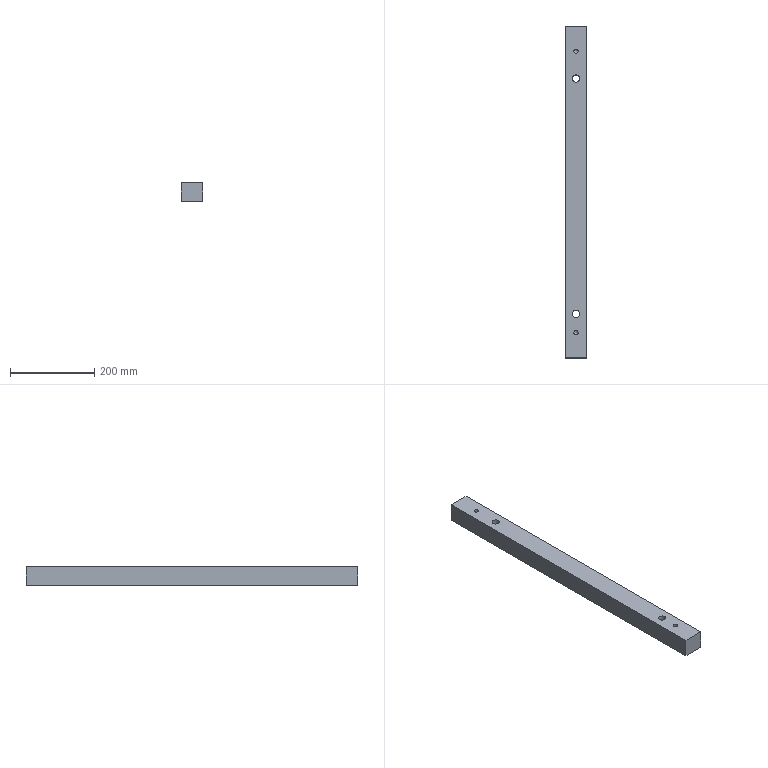Part | STEP file | 021_id2210_x_t | 1 solid | 16 faces | box 50 x 790 x 45 mm | volume 1744458 mm3 | plane 6 | cylinder 6 | cone 4 | commonest cylinder face diameters 10.3 x2 14 x2 17 x2
STEP:
#1=CARTESIAN_POINT('',(0.,0.,0.));
#2=DIRECTION('',(0.,0.,1.));
#3=DIRECTION('',(1.,0.,0.));
#4=AXIS2_PLACEMENT_3D('',#1,#2,#3);
#5=CARTESIAN_POINT('',(328.5,395.,185.));
#6=VERTEX_POINT('',#5);
#7=CARTESIAN_POINT('',(378.5,395.,185.));
#8=VERTEX_POINT('',#7);
#9=CARTESIAN_POINT('',(533.5,395.,185.));
#10=DIRECTION('',(1.,0.,0.));
#11=VECTOR('',#10,1.);
#12=LINE('',#9,#11);
#13=CARTESIAN_POINT('',(533.5,0.,185.));
#14=DIRECTION('',(0.,0.,-1.));
#15=DIRECTION('',(1.,0.,0.));
#16=AXIS2_PLACEMENT_3D('',#13,#14,#15);
#17=PLANE('',#16);
#18=CARTESIAN_POINT('',(0.,-395.));
#19=DIRECTION('',(1.,0.));
#20=VECTOR('',#19,1.);
#21=LINE('',#18,#20);
#22=(GEOMETRIC_REPRESENTATION_CONTEXT(2)PARAMETRIC_REPRESENTATION_CONTEXT()REPRESENTATION_CONTEXT('',''));
#23=DEFINITIONAL_REPRESENTATION('',(#21),#22);
#24=PCURVE('',#17,#23);
#25=CARTESIAN_POINT('',(328.5,395.,-28.5));
#26=DIRECTION('',(0.,1.,0.));
#27=DIRECTION('',(0.,0.,-1.));
#28=AXIS2_PLACEMENT_3D('',#25,#26,#27);
#29=PLANE('',#28);
#30=CARTESIAN_POINT('',(-213.5,-205.));
#31=DIRECTION('',(0.,-1.));
#32=VECTOR('',#31,1.);
#33=LINE('',#30,#32);
#34=(GEOMETRIC_REPRESENTATION_CONTEXT(2)PARAMETRIC_REPRESENTATION_CONTEXT()REPRESENTATION_CONTEXT('',''));
#35=DEFINITIONAL_REPRESENTATION('',(#33),#34);
#36=PCURVE('',#29,#35);
#37=SURFACE_CURVE('',#12,(#24,#36),.PCURVE_S1.);
#38=EDGE_CURVE('',#6,#8,#37,.T.);
#39=ORIENTED_EDGE('',*,*,#38,.T.);
#40=CARTESIAN_POINT('',(378.5,-395.,185.));
#41=VERTEX_POINT('',#40);
#42=CARTESIAN_POINT('',(378.5,-210.,185.));
#43=DIRECTION('',(0.,-1.,0.));
#44=VECTOR('',#43,1.);
#45=LINE('',#42,#44);
#46=CARTESIAN_POINT('',(-155.,210.));
#47=DIRECTION('',(0.,1.));
#48=VECTOR('',#47,1.);
#49=LINE('',#46,#48);
#50=(GEOMETRIC_REPRESENTATION_CONTEXT(2)PARAMETRIC_REPRESENTATION_CONTEXT()REPRESENTATION_CONTEXT('',''));
#51=DEFINITIONAL_REPRESENTATION('',(#49),#50);
#52=PCURVE('',#17,#51);
#53=CARTESIAN_POINT('',(378.5,-210.,-28.5));
#54=DIRECTION('',(-1.,0.,0.));
#55=DIRECTION('',(0.,0.,1.));
#56=AXIS2_PLACEMENT_3D('',#53,#54,#55);
#57=PLANE('',#56);
#58=CARTESIAN_POINT('',(213.5,0.));
#59=DIRECTION('',(0.,-1.));
#60=VECTOR('',#59,1.);
#61=LINE('',#58,#60);
#62=(GEOMETRIC_REPRESENTATION_CONTEXT(2)PARAMETRIC_REPRESENTATION_CONTEXT()REPRESENTATION_CONTEXT('',''));
#63=DEFINITIONAL_REPRESENTATION('',(#61),#62);
#64=PCURVE('',#57,#63);
#65=SURFACE_CURVE('',#45,(#52,#64),.PCURVE_S1.);
#66=EDGE_CURVE('',#8,#41,#65,.T.);
#67=ORIENTED_EDGE('',*,*,#66,.T.);
#68=CARTESIAN_POINT('',(328.5,-395.,185.));
#69=VERTEX_POINT('',#68);
#70=CARTESIAN_POINT('',(533.5,-395.,185.));
#71=DIRECTION('',(1.,0.,0.));
#72=VECTOR('',#71,1.);
#73=LINE('',#70,#72);
#74=CARTESIAN_POINT('',(0.,395.));
#75=DIRECTION('',(1.,0.));
#76=VECTOR('',#75,1.);
#77=LINE('',#74,#76);
#78=(GEOMETRIC_REPRESENTATION_CONTEXT(2)PARAMETRIC_REPRESENTATION_CONTEXT()REPRESENTATION_CONTEXT('',''));
#79=DEFINITIONAL_REPRESENTATION('',(#77),#78);
#80=PCURVE('',#17,#79);
#81=CARTESIAN_POINT('',(328.5,-395.,-28.5));
#82=DIRECTION('',(0.,1.,0.));
#83=DIRECTION('',(0.,0.,-1.));
#84=AXIS2_PLACEMENT_3D('',#81,#82,#83);
#85=PLANE('',#84);
#86=CARTESIAN_POINT('',(-213.5,-205.));
#87=DIRECTION('',(0.,-1.));
#88=VECTOR('',#87,1.);
#89=LINE('',#86,#88);
#90=(GEOMETRIC_REPRESENTATION_CONTEXT(2)PARAMETRIC_REPRESENTATION_CONTEXT()REPRESENTATION_CONTEXT('',''));
#91=DEFINITIONAL_REPRESENTATION('',(#89),#90);
#92=PCURVE('',#85,#91);
#93=SURFACE_CURVE('',#73,(#80,#92),.PCURVE_S1.);
#94=EDGE_CURVE('',#69,#41,#93,.T.);
#95=ORIENTED_EDGE('',*,*,#94,.F.);
#96=CARTESIAN_POINT('',(328.5,0.,185.));
#97=DIRECTION('',(0.,1.,0.));
#98=VECTOR('',#97,1.);
#99=LINE('',#96,#98);
#100=CARTESIAN_POINT('',(-205.,0.));
#101=DIRECTION('',(0.,-1.));
#102=VECTOR('',#101,1.);
#103=LINE('',#100,#102);
#104=(GEOMETRIC_REPRESENTATION_CONTEXT(2)PARAMETRIC_REPRESENTATION_CONTEXT()REPRESENTATION_CONTEXT('',''));
#105=DEFINITIONAL_REPRESENTATION('',(#103),#104);
#106=PCURVE('',#17,#105);
#107=CARTESIAN_POINT('',(328.5,-210.,-28.5));
#108=DIRECTION('',(-1.,0.,0.));
#109=DIRECTION('',(0.,0.,1.));
#110=AXIS2_PLACEMENT_3D('',#107,#108,#109);
#111=PLANE('',#110);
#112=CARTESIAN_POINT('',(213.5,210.));
#113=DIRECTION('',(0.,1.));
#114=VECTOR('',#113,1.);
#115=LINE('',#112,#114);
#116=(GEOMETRIC_REPRESENTATION_CONTEXT(2)PARAMETRIC_REPRESENTATION_CONTEXT()REPRESENTATION_CONTEXT('',''));
#117=DEFINITIONAL_REPRESENTATION('',(#115),#116);
#118=PCURVE('',#111,#117);
#119=SURFACE_CURVE('',#99,(#106,#118),.PCURVE_S1.);
#120=EDGE_CURVE('',#69,#6,#119,.T.);
#121=ORIENTED_EDGE('',*,*,#120,.T.);
#122=EDGE_LOOP('',(#39,#67,#95,#121));
#123=FACE_BOUND('',#122,.T.);
#124=CARTESIAN_POINT('',(346.5,-370.,185.));
#125=VERTEX_POINT('',#124);
#126=CARTESIAN_POINT('',(360.5,-370.,185.));
#127=VERTEX_POINT('',#126);
#128=CARTESIAN_POINT('',(353.5,-370.,185.));
#129=DIRECTION('',(0.,0.,1.));
#130=DIRECTION('',(-1.,0.,0.));
#131=AXIS2_PLACEMENT_3D('',#128,#129,#130);
#132=CIRCLE('',#131,7.);
#133=CARTESIAN_POINT('',(-187.,370.));
#134=CARTESIAN_POINT('',(-187.,382.124));
#135=CARTESIAN_POINT('',(-176.5,376.062));
#136=CARTESIAN_POINT('',(-166.,370.));
#137=CARTESIAN_POINT('',(-176.5,363.938));
#138=CARTESIAN_POINT('',(-187.,357.876));
#139=CARTESIAN_POINT('',(-187.,370.));
#140=(BOUNDED_CURVE()B_SPLINE_CURVE(2,(#133,#134,#135,#136,#137,#138,#139),.UNSPECIFIED.,.T.,.F.)B_SPLINE_CURVE_WITH_KNOTS((1,2,2,2,2,1),(-2.094,0.,2.094,4.189,6.283,8.378),.UNSPECIFIED.)CURVE()GEOMETRIC_REPRESENTATION_ITEM()RATIONAL_B_SPLINE_CURVE((1.,0.5,1.,0.5,1.,0.5,1.))REPRESENTATION_ITEM(''));
#141=(GEOMETRIC_REPRESENTATION_CONTEXT(2)PARAMETRIC_REPRESENTATION_CONTEXT()REPRESENTATION_CONTEXT('',''));
#142=DEFINITIONAL_REPRESENTATION('',(#140),#141);
#143=PCURVE('',#17,#142);
#144=CARTESIAN_POINT('',(353.5,-370.,121.));
#145=DIRECTION('',(0.,0.,1.));
#146=DIRECTION('',(1.,0.,0.));
#147=AXIS2_PLACEMENT_3D('',#144,#145,#146);
#148=CYLINDRICAL_SURFACE('',#147,7.);
#149=CARTESIAN_POINT('',(3.142,64.));
#150=DIRECTION('',(1.,0.));
#151=VECTOR('',#150,1.);
#152=LINE('',#149,#151);
#153=(GEOMETRIC_REPRESENTATION_CONTEXT(2)PARAMETRIC_REPRESENTATION_CONTEXT()REPRESENTATION_CONTEXT('',''));
#154=DEFINITIONAL_REPRESENTATION('',(#152),#153);
#155=PCURVE('',#148,#154);
#156=SURFACE_CURVE('',#132,(#143,#155),.PCURVE_S1.);
#157=EDGE_CURVE('',#125,#127,#156,.T.);
#158=ORIENTED_EDGE('',*,*,#157,.T.);
#159=CARTESIAN_POINT('',(353.5,-370.,185.));
#160=DIRECTION('',(0.,0.,1.));
#161=DIRECTION('',(-1.,0.,0.));
#162=AXIS2_PLACEMENT_3D('',#159,#160,#161);
#163=CIRCLE('',#162,7.);
#164=CARTESIAN_POINT('',(-187.,370.));
#165=CARTESIAN_POINT('',(-187.,382.124));
#166=CARTESIAN_POINT('',(-176.5,376.062));
#167=CARTESIAN_POINT('',(-166.,370.));
#168=CARTESIAN_POINT('',(-176.5,363.938));
#169=CARTESIAN_POINT('',(-187.,357.876));
#170=CARTESIAN_POINT('',(-187.,370.));
#171=(BOUNDED_CURVE()B_SPLINE_CURVE(2,(#164,#165,#166,#167,#168,#169,#170),.UNSPECIFIED.,.T.,.F.)B_SPLINE_CURVE_WITH_KNOTS((1,2,2,2,2,1),(-2.094,0.,2.094,4.189,6.283,8.378),.UNSPECIFIED.)CURVE()GEOMETRIC_REPRESENTATION_ITEM()RATIONAL_B_SPLINE_CURVE((1.,0.5,1.,0.5,1.,0.5,1.))REPRESENTATION_ITEM(''));
#172=(GEOMETRIC_REPRESENTATION_CONTEXT(2)PARAMETRIC_REPRESENTATION_CONTEXT()REPRESENTATION_CONTEXT('',''));
#173=DEFINITIONAL_REPRESENTATION('',(#171),#172);
#174=PCURVE('',#17,#173);
#175=CARTESIAN_POINT('',(-3.142,64.));
#176=DIRECTION('',(1.,0.));
#177=VECTOR('',#176,1.);
#178=LINE('',#175,#177);
#179=(GEOMETRIC_REPRESENTATION_CONTEXT(2)PARAMETRIC_REPRESENTATION_CONTEXT()REPRESENTATION_CONTEXT('',''));
#180=DEFINITIONAL_REPRESENTATION('',(#178),#179);
#181=PCURVE('',#148,#180);
#182=SURFACE_CURVE('',#163,(#174,#181),.PCURVE_S1.);
#183=EDGE_CURVE('',#127,#125,#182,.T.);
#184=ORIENTED_EDGE('',*,*,#183,.T.);
#185=EDGE_LOOP('',(#158,#184));
#186=FACE_BOUND('',#185,.T.);
#187=CARTESIAN_POINT('',(346.5,370.,185.));
#188=VERTEX_POINT('',#187);
#189=CARTESIAN_POINT('',(360.5,370.,185.));
#190=VERTEX_POINT('',#189);
#191=CARTESIAN_POINT('',(353.5,370.,185.));
#192=DIRECTION('',(0.,0.,-1.));
#193=DIRECTION('',(-1.,0.,0.));
#194=AXIS2_PLACEMENT_3D('',#191,#192,#193);
#195=CIRCLE('',#194,7.);
#196=CARTESIAN_POINT('',(-180.,-370.));
#197=DIRECTION('',(-1.,0.));
#198=AXIS2_PLACEMENT_2D('',#196,#197);
#199=CIRCLE('',#198,7.);
#200=(GEOMETRIC_REPRESENTATION_CONTEXT(2)PARAMETRIC_REPRESENTATION_CONTEXT()REPRESENTATION_CONTEXT('',''));
#201=DEFINITIONAL_REPRESENTATION('',(#199),#200);
#202=PCURVE('',#17,#201);
#203=CARTESIAN_POINT('',(353.5,370.,121.));
#204=DIRECTION('',(0.,0.,1.));
#205=DIRECTION('',(1.,0.,0.));
#206=AXIS2_PLACEMENT_3D('',#203,#204,#205);
#207=CYLINDRICAL_SURFACE('',#206,7.);
#208=CARTESIAN_POINT('',(3.142,64.));
#209=DIRECTION('',(-1.,0.));
#210=VECTOR('',#209,1.);
#211=LINE('',#208,#210);
#212=(GEOMETRIC_REPRESENTATION_CONTEXT(2)PARAMETRIC_REPRESENTATION_CONTEXT()REPRESENTATION_CONTEXT('',''));
#213=DEFINITIONAL_REPRESENTATION('',(#211),#212);
#214=PCURVE('',#207,#213);
#215=SURFACE_CURVE('',#195,(#202,#214),.PCURVE_S1.);
#216=EDGE_CURVE('',#188,#190,#215,.T.);
#217=ORIENTED_EDGE('',*,*,#216,.F.);
#218=CARTESIAN_POINT('',(353.5,370.,185.));
#219=DIRECTION('',(0.,0.,-1.));
#220=DIRECTION('',(-1.,0.,0.));
#221=AXIS2_PLACEMENT_3D('',#218,#219,#220);
#222=CIRCLE('',#221,7.);
#223=CARTESIAN_POINT('',(-180.,-370.));
#224=DIRECTION('',(-1.,0.));
#225=AXIS2_PLACEMENT_2D('',#223,#224);
#226=CIRCLE('',#225,7.);
#227=(GEOMETRIC_REPRESENTATION_CONTEXT(2)PARAMETRIC_REPRESENTATION_CONTEXT()REPRESENTATION_CONTEXT('',''));
#228=DEFINITIONAL_REPRESENTATION('',(#226),#227);
#229=PCURVE('',#17,#228);
#230=CARTESIAN_POINT('',(9.425,64.));
#231=DIRECTION('',(-1.,0.));
#232=VECTOR('',#231,1.);
#233=LINE('',#230,#232);
#234=(GEOMETRIC_REPRESENTATION_CONTEXT(2)PARAMETRIC_REPRESENTATION_CONTEXT()REPRESENTATION_CONTEXT('',''));
#235=DEFINITIONAL_REPRESENTATION('',(#233),#234);
#236=PCURVE('',#207,#235);
#237=SURFACE_CURVE('',#222,(#229,#236),.PCURVE_S1.);
#238=EDGE_CURVE('',#190,#188,#237,.T.);
#239=ORIENTED_EDGE('',*,*,#238,.F.);
#240=EDGE_LOOP('',(#217,#239));
#241=FACE_BOUND('',#240,.T.);
#242=CARTESIAN_POINT('',(345.,-290.,185.));
#243=VERTEX_POINT('',#242);
#244=CARTESIAN_POINT('',(353.5,-290.,185.));
#245=DIRECTION('',(0.,0.,-1.));
#246=DIRECTION('',(-1.,0.,0.));
#247=AXIS2_PLACEMENT_3D('',#244,#245,#246);
#248=CIRCLE('',#247,8.5);
#249=CARTESIAN_POINT('',(-180.,290.));
#250=DIRECTION('',(-1.,0.));
#251=AXIS2_PLACEMENT_2D('',#249,#250);
#252=CIRCLE('',#251,8.5);
#253=(GEOMETRIC_REPRESENTATION_CONTEXT(2)PARAMETRIC_REPRESENTATION_CONTEXT()REPRESENTATION_CONTEXT('',''));
#254=DEFINITIONAL_REPRESENTATION('',(#252),#253);
#255=PCURVE('',#17,#254);
#256=CARTESIAN_POINT('',(353.5,-290.,150.016));
#257=DIRECTION('',(0.,0.,1.));
#258=DIRECTION('',(1.,0.,0.));
#259=AXIS2_PLACEMENT_3D('',#256,#257,#258);
#260=CYLINDRICAL_SURFACE('',#259,8.5);
#261=CARTESIAN_POINT('',(9.425,34.984));
#262=DIRECTION('',(-1.,0.));
#263=VECTOR('',#262,1.);
#264=LINE('',#261,#263);
#265=(GEOMETRIC_REPRESENTATION_CONTEXT(2)PARAMETRIC_REPRESENTATION_CONTEXT()REPRESENTATION_CONTEXT('',''));
#266=DEFINITIONAL_REPRESENTATION('',(#264),#265);
#267=PCURVE('',#260,#266);
#268=SURFACE_CURVE('',#248,(#255,#267),.PCURVE_S1.);
#269=EDGE_CURVE('',#243,#243,#268,.T.);
#270=ORIENTED_EDGE('',*,*,#269,.F.);
#271=EDGE_LOOP('',(#270));
#272=FACE_BOUND('',#271,.T.);
#273=CARTESIAN_POINT('',(345.,270.,185.));
#274=VERTEX_POINT('',#273);
#275=CARTESIAN_POINT('',(353.5,270.,185.));
#276=DIRECTION('',(0.,0.,1.));
#277=DIRECTION('',(-1.,0.,0.));
#278=AXIS2_PLACEMENT_3D('',#275,#276,#277);
#279=CIRCLE('',#278,8.5);
#280=CARTESIAN_POINT('',(-188.5,-270.));
#281=CARTESIAN_POINT('',(-188.5,-255.278));
#282=CARTESIAN_POINT('',(-175.75,-262.639));
#283=CARTESIAN_POINT('',(-163.,-270.));
#284=CARTESIAN_POINT('',(-175.75,-277.361));
#285=CARTESIAN_POINT('',(-188.5,-284.722));
#286=CARTESIAN_POINT('',(-188.5,-270.));
#287=(BOUNDED_CURVE()B_SPLINE_CURVE(2,(#280,#281,#282,#283,#284,#285,#286),.UNSPECIFIED.,.T.,.F.)B_SPLINE_CURVE_WITH_KNOTS((1,2,2,2,2,1),(-2.094,0.,2.094,4.189,6.283,8.378),.UNSPECIFIED.)CURVE()GEOMETRIC_REPRESENTATION_ITEM()RATIONAL_B_SPLINE_CURVE((1.,0.5,1.,0.5,1.,0.5,1.))REPRESENTATION_ITEM(''));
#288=(GEOMETRIC_REPRESENTATION_CONTEXT(2)PARAMETRIC_REPRESENTATION_CONTEXT()REPRESENTATION_CONTEXT('',''));
#289=DEFINITIONAL_REPRESENTATION('',(#287),#288);
#290=PCURVE('',#17,#289);
#291=CARTESIAN_POINT('',(353.5,270.,150.016));
#292=DIRECTION('',(0.,0.,1.));
#293=DIRECTION('',(1.,0.,0.));
#294=AXIS2_PLACEMENT_3D('',#291,#292,#293);
#295=CYLINDRICAL_SURFACE('',#294,8.5);
#296=CARTESIAN_POINT('',(3.142,34.984));
#297=DIRECTION('',(1.,0.));
#298=VECTOR('',#297,1.);
#299=LINE('',#296,#298);
#300=(GEOMETRIC_REPRESENTATION_CONTEXT(2)PARAMETRIC_REPRESENTATION_CONTEXT()REPRESENTATION_CONTEXT('',''));
#301=DEFINITIONAL_REPRESENTATION('',(#299),#300);
#302=PCURVE('',#295,#301);
#303=SURFACE_CURVE('',#279,(#290,#302),.PCURVE_S1.);
#304=EDGE_CURVE('',#274,#274,#303,.T.);
#305=ORIENTED_EDGE('',*,*,#304,.T.);
#306=EDGE_LOOP('',(#305));
#307=FACE_BOUND('',#306,.T.);
#308=ADVANCED_FACE('',(#123,#186,#241,#272,#307),#17,.T.);
#309=CARTESIAN_POINT('',(348.35,-335.,230.));
#310=VERTEX_POINT('',#309);
#311=CARTESIAN_POINT('',(353.5,-335.,230.));
#312=DIRECTION('',(0.,0.,-1.));
#313=DIRECTION('',(-1.,0.,0.));
#314=AXIS2_PLACEMENT_3D('',#311,#312,#313);
#315=CIRCLE('',#314,5.15);
#316=CARTESIAN_POINT('',(328.5,-210.,230.));
#317=DIRECTION('',(0.,0.,-1.));
#318=DIRECTION('',(0.,-1.,0.));
#319=AXIS2_PLACEMENT_3D('',#316,#317,#318);
#320=PLANE('',#319);
#321=CARTESIAN_POINT('',(125.,-25.));
#322=DIRECTION('',(0.,1.));
#323=AXIS2_PLACEMENT_2D('',#321,#322);
#324=CIRCLE('',#323,5.15);
#325=(GEOMETRIC_REPRESENTATION_CONTEXT(2)PARAMETRIC_REPRESENTATION_CONTEXT()REPRESENTATION_CONTEXT('',''));
#326=DEFINITIONAL_REPRESENTATION('',(#324),#325);
#327=PCURVE('',#320,#326);
#328=CARTESIAN_POINT('',(353.5,-335.,259.));
#329=DIRECTION('',(0.,0.,-1.));
#330=DIRECTION('',(-1.,0.,0.));
#331=AXIS2_PLACEMENT_3D('',#328,#329,#330);
#332=CYLINDRICAL_SURFACE('',#331,5.15);
#333=CARTESIAN_POINT('',(0.,29.));
#334=DIRECTION('',(1.,0.));
#335=VECTOR('',#334,1.);
#336=LINE('',#333,#335);
#337=(GEOMETRIC_REPRESENTATION_CONTEXT(2)PARAMETRIC_REPRESENTATION_CONTEXT()REPRESENTATION_CONTEXT('',''));
#338=DEFINITIONAL_REPRESENTATION('',(#336),#337);
#339=PCURVE('',#332,#338);
#340=SURFACE_CURVE('',#315,(#327,#339),.PCURVE_S1.);
#341=EDGE_CURVE('',#310,#310,#340,.T.);
#342=ORIENTED_EDGE('',*,*,#341,.T.);
#343=EDGE_LOOP('',(#342));
#344=FACE_BOUND('',#343,.T.);
#345=CARTESIAN_POINT('',(348.35,335.,230.));
#346=VERTEX_POINT('',#345);
#347=CARTESIAN_POINT('',(353.5,335.,230.));
#348=DIRECTION('',(0.,0.,1.));
#349=DIRECTION('',(-1.,0.,0.));
#350=AXIS2_PLACEMENT_3D('',#347,#348,#349);
#351=CIRCLE('',#350,5.15);
#352=CARTESIAN_POINT('',(-545.,-19.85));
#353=CARTESIAN_POINT('',(-536.08,-19.85));
#354=CARTESIAN_POINT('',(-540.54,-27.575));
#355=CARTESIAN_POINT('',(-545.,-35.3));
#356=CARTESIAN_POINT('',(-549.46,-27.575));
#357=CARTESIAN_POINT('',(-553.92,-19.85));
#358=CARTESIAN_POINT('',(-545.,-19.85));
#359=(BOUNDED_CURVE()B_SPLINE_CURVE(2,(#352,#353,#354,#355,#356,#357,#358),.UNSPECIFIED.,.T.,.F.)B_SPLINE_CURVE_WITH_KNOTS((1,2,2,2,2,1),(-2.094,0.,2.094,4.189,6.283,8.378),.UNSPECIFIED.)CURVE()GEOMETRIC_REPRESENTATION_ITEM()RATIONAL_B_SPLINE_CURVE((1.,0.5,1.,0.5,1.,0.5,1.))REPRESENTATION_ITEM(''));
#360=(GEOMETRIC_REPRESENTATION_CONTEXT(2)PARAMETRIC_REPRESENTATION_CONTEXT()REPRESENTATION_CONTEXT('',''));
#361=DEFINITIONAL_REPRESENTATION('',(#359),#360);
#362=PCURVE('',#320,#361);
#363=CARTESIAN_POINT('',(353.5,335.,259.));
#364=DIRECTION('',(0.,0.,-1.));
#365=DIRECTION('',(-1.,0.,0.));
#366=AXIS2_PLACEMENT_3D('',#363,#364,#365);
#367=CYLINDRICAL_SURFACE('',#366,5.15);
#368=CARTESIAN_POINT('',(6.283,29.));
#369=DIRECTION('',(-1.,0.));
#370=VECTOR('',#369,1.);
#371=LINE('',#368,#370);
#372=(GEOMETRIC_REPRESENTATION_CONTEXT(2)PARAMETRIC_REPRESENTATION_CONTEXT()REPRESENTATION_CONTEXT('',''));
#373=DEFINITIONAL_REPRESENTATION('',(#371),#372);
#374=PCURVE('',#367,#373);
#375=SURFACE_CURVE('',#351,(#362,#374),.PCURVE_S1.);
#376=EDGE_CURVE('',#346,#346,#375,.T.);
#377=ORIENTED_EDGE('',*,*,#376,.F.);
#378=EDGE_LOOP('',(#377));
#379=FACE_BOUND('',#378,.T.);
#380=CARTESIAN_POINT('',(345.,270.,230.));
#381=VERTEX_POINT('',#380);
#382=CARTESIAN_POINT('',(353.5,270.,230.));
#383=DIRECTION('',(0.,0.,1.));
#384=DIRECTION('',(-1.,0.,0.));
#385=AXIS2_PLACEMENT_3D('',#382,#383,#384);
#386=CIRCLE('',#385,8.5);
#387=CARTESIAN_POINT('',(-480.,-16.5));
#388=CARTESIAN_POINT('',(-465.278,-16.5));
#389=CARTESIAN_POINT('',(-472.639,-29.25));
#390=CARTESIAN_POINT('',(-480.,-42.));
#391=CARTESIAN_POINT('',(-487.361,-29.25));
#392=CARTESIAN_POINT('',(-494.722,-16.5));
#393=CARTESIAN_POINT('',(-480.,-16.5));
#394=(BOUNDED_CURVE()B_SPLINE_CURVE(2,(#387,#388,#389,#390,#391,#392,#393),.UNSPECIFIED.,.T.,.F.)B_SPLINE_CURVE_WITH_KNOTS((1,2,2,2,2,1),(-2.094,0.,2.094,4.189,6.283,8.378),.UNSPECIFIED.)CURVE()GEOMETRIC_REPRESENTATION_ITEM()RATIONAL_B_SPLINE_CURVE((1.,0.5,1.,0.5,1.,0.5,1.))REPRESENTATION_ITEM(''));
#395=(GEOMETRIC_REPRESENTATION_CONTEXT(2)PARAMETRIC_REPRESENTATION_CONTEXT()REPRESENTATION_CONTEXT('',''));
#396=DEFINITIONAL_REPRESENTATION('',(#394),#395);
#397=PCURVE('',#320,#396);
#398=CARTESIAN_POINT('',(3.142,79.984));
#399=DIRECTION('',(1.,0.));
#400=VECTOR('',#399,1.);
#401=LINE('',#398,#400);
#402=(GEOMETRIC_REPRESENTATION_CONTEXT(2)PARAMETRIC_REPRESENTATION_CONTEXT()REPRESENTATION_CONTEXT('',''));
#403=DEFINITIONAL_REPRESENTATION('',(#401),#402);
#404=PCURVE('',#295,#403);
#405=SURFACE_CURVE('',#386,(#397,#404),.PCURVE_S1.);
#406=EDGE_CURVE('',#381,#381,#405,.T.);
#407=ORIENTED_EDGE('',*,*,#406,.F.);
#408=EDGE_LOOP('',(#407));
#409=FACE_BOUND('',#408,.T.);
#410=CARTESIAN_POINT('',(345.,-290.,230.));
#411=VERTEX_POINT('',#410);
#412=CARTESIAN_POINT('',(353.5,-290.,230.));
#413=DIRECTION('',(0.,0.,-1.));
#414=DIRECTION('',(-1.,0.,0.));
#415=AXIS2_PLACEMENT_3D('',#412,#413,#414);
#416=CIRCLE('',#415,8.5);
#417=CARTESIAN_POINT('',(80.,-25.));
#418=DIRECTION('',(0.,1.));
#419=AXIS2_PLACEMENT_2D('',#417,#418);
#420=CIRCLE('',#419,8.5);
#421=(GEOMETRIC_REPRESENTATION_CONTEXT(2)PARAMETRIC_REPRESENTATION_CONTEXT()REPRESENTATION_CONTEXT('',''));
#422=DEFINITIONAL_REPRESENTATION('',(#420),#421);
#423=PCURVE('',#320,#422);
#424=CARTESIAN_POINT('',(9.425,79.984));
#425=DIRECTION('',(-1.,0.));
#426=VECTOR('',#425,1.);
#427=LINE('',#424,#426);
#428=(GEOMETRIC_REPRESENTATION_CONTEXT(2)PARAMETRIC_REPRESENTATION_CONTEXT()REPRESENTATION_CONTEXT('',''));
#429=DEFINITIONAL_REPRESENTATION('',(#427),#428);
#430=PCURVE('',#260,#429);
#431=SURFACE_CURVE('',#416,(#423,#430),.PCURVE_S1.);
#432=EDGE_CURVE('',#411,#411,#431,.T.);
#433=ORIENTED_EDGE('',*,*,#432,.T.);
#434=EDGE_LOOP('',(#433));
#435=FACE_BOUND('',#434,.T.);
#436=CARTESIAN_POINT('',(328.5,-395.,230.));
#437=VERTEX_POINT('',#436);
#438=CARTESIAN_POINT('',(378.5,-395.,230.));
#439=VERTEX_POINT('',#438);
#440=CARTESIAN_POINT('',(328.5,-395.,230.));
#441=DIRECTION('',(1.,0.,0.));
#442=VECTOR('',#441,1.);
#443=LINE('',#440,#442);
#444=CARTESIAN_POINT('',(185.,0.));
#445=DIRECTION('',(0.,-1.));
#446=VECTOR('',#445,1.);
#447=LINE('',#444,#446);
#448=(GEOMETRIC_REPRESENTATION_CONTEXT(2)PARAMETRIC_REPRESENTATION_CONTEXT()REPRESENTATION_CONTEXT('',''));
#449=DEFINITIONAL_REPRESENTATION('',(#447),#448);
#450=PCURVE('',#320,#449);
#451=CARTESIAN_POINT('',(-258.5,0.));
#452=DIRECTION('',(0.,-1.));
#453=VECTOR('',#452,1.);
#454=LINE('',#451,#453);
#455=(GEOMETRIC_REPRESENTATION_CONTEXT(2)PARAMETRIC_REPRESENTATION_CONTEXT()REPRESENTATION_CONTEXT('',''));
#456=DEFINITIONAL_REPRESENTATION('',(#454),#455);
#457=PCURVE('',#85,#456);
#458=SURFACE_CURVE('',#443,(#450,#457),.PCURVE_S1.);
#459=EDGE_CURVE('',#437,#439,#458,.T.);
#460=ORIENTED_EDGE('',*,*,#459,.T.);
#461=CARTESIAN_POINT('',(378.5,395.,230.));
#462=VERTEX_POINT('',#461);
#463=CARTESIAN_POINT('',(378.5,-210.,230.));
#464=DIRECTION('',(0.,-1.,0.));
#465=VECTOR('',#464,1.);
#466=LINE('',#463,#465);
#467=CARTESIAN_POINT('',(0.,-50.));
#468=DIRECTION('',(1.,0.));
#469=VECTOR('',#468,1.);
#470=LINE('',#467,#469);
#471=(GEOMETRIC_REPRESENTATION_CONTEXT(2)PARAMETRIC_REPRESENTATION_CONTEXT()REPRESENTATION_CONTEXT('',''));
#472=DEFINITIONAL_REPRESENTATION('',(#470),#471);
#473=PCURVE('',#320,#472);
#474=CARTESIAN_POINT('',(258.5,0.));
#475=DIRECTION('',(0.,-1.));
#476=VECTOR('',#475,1.);
#477=LINE('',#474,#476);
#478=(GEOMETRIC_REPRESENTATION_CONTEXT(2)PARAMETRIC_REPRESENTATION_CONTEXT()REPRESENTATION_CONTEXT('',''));
#479=DEFINITIONAL_REPRESENTATION('',(#477),#478);
#480=PCURVE('',#57,#479);
#481=SURFACE_CURVE('',#466,(#473,#480),.PCURVE_S1.);
#482=EDGE_CURVE('',#462,#439,#481,.T.);
#483=ORIENTED_EDGE('',*,*,#482,.F.);
#484=CARTESIAN_POINT('',(328.5,395.,230.));
#485=VERTEX_POINT('',#484);
#486=CARTESIAN_POINT('',(328.5,395.,230.));
#487=DIRECTION('',(1.,0.,0.));
#488=VECTOR('',#487,1.);
#489=LINE('',#486,#488);
#490=CARTESIAN_POINT('',(-605.,0.));
#491=DIRECTION('',(0.,-1.));
#492=VECTOR('',#491,1.);
#493=LINE('',#490,#492);
#494=(GEOMETRIC_REPRESENTATION_CONTEXT(2)PARAMETRIC_REPRESENTATION_CONTEXT()REPRESENTATION_CONTEXT('',''));
#495=DEFINITIONAL_REPRESENTATION('',(#493),#494);
#496=PCURVE('',#320,#495);
#497=CARTESIAN_POINT('',(-258.5,0.));
#498=DIRECTION('',(0.,-1.));
#499=VECTOR('',#498,1.);
#500=LINE('',#497,#499);
#501=(GEOMETRIC_REPRESENTATION_CONTEXT(2)PARAMETRIC_REPRESENTATION_CONTEXT()REPRESENTATION_CONTEXT('',''));
#502=DEFINITIONAL_REPRESENTATION('',(#500),#501);
#503=PCURVE('',#29,#502);
#504=SURFACE_CURVE('',#489,(#496,#503),.PCURVE_S1.);
#505=EDGE_CURVE('',#485,#462,#504,.T.);
#506=ORIENTED_EDGE('',*,*,#505,.F.);
#507=CARTESIAN_POINT('',(328.5,-210.,230.));
#508=DIRECTION('',(0.,-1.,0.));
#509=VECTOR('',#508,1.);
#510=LINE('',#507,#509);
#511=CARTESIAN_POINT('',(0.,0.));
#512=DIRECTION('',(1.,0.));
#513=VECTOR('',#512,1.);
#514=LINE('',#511,#513);
#515=(GEOMETRIC_REPRESENTATION_CONTEXT(2)PARAMETRIC_REPRESENTATION_CONTEXT()REPRESENTATION_CONTEXT('',''));
#516=DEFINITIONAL_REPRESENTATION('',(#514),#515);
#517=PCURVE('',#320,#516);
#518=CARTESIAN_POINT('',(258.5,0.));
#519=DIRECTION('',(0.,-1.));
#520=VECTOR('',#519,1.);
#521=LINE('',#518,#520);
#522=(GEOMETRIC_REPRESENTATION_CONTEXT(2)PARAMETRIC_REPRESENTATION_CONTEXT()REPRESENTATION_CONTEXT('',''));
#523=DEFINITIONAL_REPRESENTATION('',(#521),#522);
#524=PCURVE('',#111,#523);
#525=SURFACE_CURVE('',#510,(#517,#524),.PCURVE_S1.);
#526=EDGE_CURVE('',#485,#437,#525,.T.);
#527=ORIENTED_EDGE('',*,*,#526,.T.);
#528=EDGE_LOOP('',(#460,#483,#506,#527));
#529=FACE_BOUND('',#528,.T.);
#530=ADVANCED_FACE('',(#344,#379,#409,#435,#529),#320,.F.);
#531=ORIENTED_EDGE('',*,*,#66,.F.);
#532=CARTESIAN_POINT('',(378.5,395.,-28.5));
#533=DIRECTION('',(0.,0.,1.));
#534=VECTOR('',#533,1.);
#535=LINE('',#532,#534);
#536=CARTESIAN_POINT('',(0.,605.));
#537=DIRECTION('',(1.,0.));
#538=VECTOR('',#537,1.);
#539=LINE('',#536,#538);
#540=(GEOMETRIC_REPRESENTATION_CONTEXT(2)PARAMETRIC_REPRESENTATION_CONTEXT()REPRESENTATION_CONTEXT('',''));
#541=DEFINITIONAL_REPRESENTATION('',(#539),#540);
#542=PCURVE('',#57,#541);
#543=CARTESIAN_POINT('',(0.,-50.));
#544=DIRECTION('',(-1.,0.));
#545=VECTOR('',#544,1.);
#546=LINE('',#543,#545);
#547=(GEOMETRIC_REPRESENTATION_CONTEXT(2)PARAMETRIC_REPRESENTATION_CONTEXT()REPRESENTATION_CONTEXT('',''));
#548=DEFINITIONAL_REPRESENTATION('',(#546),#547);
#549=PCURVE('',#29,#548);
#550=SURFACE_CURVE('',#535,(#542,#549),.PCURVE_S1.);
#551=EDGE_CURVE('',#8,#462,#550,.T.);
#552=ORIENTED_EDGE('',*,*,#551,.T.);
#553=ORIENTED_EDGE('',*,*,#482,.T.);
#554=CARTESIAN_POINT('',(378.5,-395.,-28.5));
#555=DIRECTION('',(0.,0.,-1.));
#556=VECTOR('',#555,1.);
#557=LINE('',#554,#556);
#558=CARTESIAN_POINT('',(0.,-185.));
#559=DIRECTION('',(-1.,0.));
#560=VECTOR('',#559,1.);
#561=LINE('',#558,#560);
#562=(GEOMETRIC_REPRESENTATION_CONTEXT(2)PARAMETRIC_REPRESENTATION_CONTEXT()REPRESENTATION_CONTEXT('',''));
#563=DEFINITIONAL_REPRESENTATION('',(#561),#562);
#564=PCURVE('',#57,#563);
#565=CARTESIAN_POINT('',(0.,-50.));
#566=DIRECTION('',(1.,0.));
#567=VECTOR('',#566,1.);
#568=LINE('',#565,#567);
#569=(GEOMETRIC_REPRESENTATION_CONTEXT(2)PARAMETRIC_REPRESENTATION_CONTEXT()REPRESENTATION_CONTEXT('',''));
#570=DEFINITIONAL_REPRESENTATION('',(#568),#569);
#571=PCURVE('',#85,#570);
#572=SURFACE_CURVE('',#557,(#564,#571),.PCURVE_S1.);
#573=EDGE_CURVE('',#439,#41,#572,.T.);
#574=ORIENTED_EDGE('',*,*,#573,.T.);
#575=EDGE_LOOP('',(#531,#552,#553,#574));
#576=FACE_BOUND('',#575,.T.);
#577=ADVANCED_FACE('',(#576),#57,.F.);
#578=ORIENTED_EDGE('',*,*,#94,.T.);
#579=ORIENTED_EDGE('',*,*,#573,.F.);
#580=ORIENTED_EDGE('',*,*,#459,.F.);
#581=CARTESIAN_POINT('',(328.5,-395.,-28.5));
#582=DIRECTION('',(0.,0.,-1.));
#583=VECTOR('',#582,1.);
#584=LINE('',#581,#583);
#585=CARTESIAN_POINT('',(0.,0.));
#586=DIRECTION('',(1.,0.));
#587=VECTOR('',#586,1.);
#588=LINE('',#585,#587);
#589=(GEOMETRIC_REPRESENTATION_CONTEXT(2)PARAMETRIC_REPRESENTATION_CONTEXT()REPRESENTATION_CONTEXT('',''));
#590=DEFINITIONAL_REPRESENTATION('',(#588),#589);
#591=PCURVE('',#85,#590);
#592=CARTESIAN_POINT('',(0.,-185.));
#593=DIRECTION('',(-1.,0.));
#594=VECTOR('',#593,1.);
#595=LINE('',#592,#594);
#596=(GEOMETRIC_REPRESENTATION_CONTEXT(2)PARAMETRIC_REPRESENTATION_CONTEXT()REPRESENTATION_CONTEXT('',''));
#597=DEFINITIONAL_REPRESENTATION('',(#595),#596);
#598=PCURVE('',#111,#597);
#599=SURFACE_CURVE('',#584,(#591,#598),.PCURVE_S1.);
#600=EDGE_CURVE('',#437,#69,#599,.T.);
#601=ORIENTED_EDGE('',*,*,#600,.T.);
#602=EDGE_LOOP('',(#578,#579,#580,#601));
#603=FACE_BOUND('',#602,.T.);
#604=ADVANCED_FACE('',(#603),#85,.F.);
#605=CARTESIAN_POINT('',(328.5,395.,-28.5));
#606=DIRECTION('',(0.,0.,1.));
#607=VECTOR('',#606,1.);
#608=LINE('',#605,#607);
#609=CARTESIAN_POINT('',(0.,605.));
#610=DIRECTION('',(1.,0.));
#611=VECTOR('',#610,1.);
#612=LINE('',#609,#611);
#613=(GEOMETRIC_REPRESENTATION_CONTEXT(2)PARAMETRIC_REPRESENTATION_CONTEXT()REPRESENTATION_CONTEXT('',''));
#614=DEFINITIONAL_REPRESENTATION('',(#612),#613);
#615=PCURVE('',#111,#614);
#616=CARTESIAN_POINT('',(0.,0.));
#617=DIRECTION('',(-1.,0.));
#618=VECTOR('',#617,1.);
#619=LINE('',#616,#618);
#620=(GEOMETRIC_REPRESENTATION_CONTEXT(2)PARAMETRIC_REPRESENTATION_CONTEXT()REPRESENTATION_CONTEXT('',''));
#621=DEFINITIONAL_REPRESENTATION('',(#619),#620);
#622=PCURVE('',#29,#621);
#623=SURFACE_CURVE('',#608,(#615,#622),.PCURVE_S1.);
#624=EDGE_CURVE('',#6,#485,#623,.T.);
#625=ORIENTED_EDGE('',*,*,#624,.F.);
#626=ORIENTED_EDGE('',*,*,#120,.F.);
#627=ORIENTED_EDGE('',*,*,#600,.F.);
#628=ORIENTED_EDGE('',*,*,#526,.F.);
#629=EDGE_LOOP('',(#625,#626,#627,#628));
#630=FACE_BOUND('',#629,.T.);
#631=ADVANCED_FACE('',(#630),#111,.T.);
#632=ORIENTED_EDGE('',*,*,#551,.F.);
#633=ORIENTED_EDGE('',*,*,#38,.F.);
#634=ORIENTED_EDGE('',*,*,#624,.T.);
#635=ORIENTED_EDGE('',*,*,#505,.T.);
#636=EDGE_LOOP('',(#632,#633,#634,#635));
#637=FACE_BOUND('',#636,.T.);
#638=ADVANCED_FACE('',(#637),#29,.T.);
#639=ORIENTED_EDGE('',*,*,#238,.F.);
#640=CARTESIAN_POINT('',(360.5,370.,209.459));
#641=VERTEX_POINT('',#640);
#642=CARTESIAN_POINT('',(360.5,370.,185.));
#643=CARTESIAN_POINT('',(360.5,370.,209.459));
#644=B_SPLINE_CURVE_WITH_KNOTS('',1,(#642,#643),.UNSPECIFIED.,.F.,.F.,(2,2),(64.,88.459),.PIECEWISE_BEZIER_KNOTS.);
#645=CARTESIAN_POINT('',(6.283,0.));
#646=DIRECTION('',(0.,1.));
#647=VECTOR('',#646,1.);
#648=LINE('',#645,#647);
#649=(GEOMETRIC_REPRESENTATION_CONTEXT(2)PARAMETRIC_REPRESENTATION_CONTEXT()REPRESENTATION_CONTEXT('',''));
#650=DEFINITIONAL_REPRESENTATION('',(#648),#649);
#651=PCURVE('',#207,#650);
#652=CARTESIAN_POINT('',(0.,0.));
#653=DIRECTION('',(0.,1.));
#654=VECTOR('',#653,1.);
#655=LINE('',#652,#654);
#656=(GEOMETRIC_REPRESENTATION_CONTEXT(2)PARAMETRIC_REPRESENTATION_CONTEXT()REPRESENTATION_CONTEXT('',''));
#657=DEFINITIONAL_REPRESENTATION('',(#655),#656);
#658=PCURVE('',#207,#657);
#659=SEAM_CURVE('',#644,(#651,#658),.PCURVE_S1.);
#660=EDGE_CURVE('',#190,#641,#659,.T.);
#661=ORIENTED_EDGE('',*,*,#660,.T.);
#662=CARTESIAN_POINT('',(346.5,370.,209.459));
#663=VERTEX_POINT('',#662);
#664=CARTESIAN_POINT('',(353.5,370.,209.459));
#665=DIRECTION('',(0.,0.,-1.));
#666=DIRECTION('',(1.,0.,0.));
#667=AXIS2_PLACEMENT_3D('',#664,#665,#666);
#668=CIRCLE('',#667,7.);
#669=CARTESIAN_POINT('',(6.283,88.459));
#670=DIRECTION('',(-1.,0.));
#671=VECTOR('',#670,1.);
#672=LINE('',#669,#671);
#673=(GEOMETRIC_REPRESENTATION_CONTEXT(2)PARAMETRIC_REPRESENTATION_CONTEXT()REPRESENTATION_CONTEXT('',''));
#674=DEFINITIONAL_REPRESENTATION('',(#672),#673);
#675=PCURVE('',#207,#674);
#676=CARTESIAN_POINT('',(353.5,370.,209.459));
#677=DIRECTION('',(0.,0.,-1.));
#678=DIRECTION('',(-1.,0.,0.));
#679=AXIS2_PLACEMENT_3D('',#676,#677,#678);
#680=CONICAL_SURFACE('',#679,7.,1.047);
#681=CARTESIAN_POINT('',(3.142,0.));
#682=DIRECTION('',(1.,0.));
#683=VECTOR('',#682,1.);
#684=LINE('',#681,#683);
#685=(GEOMETRIC_REPRESENTATION_CONTEXT(2)PARAMETRIC_REPRESENTATION_CONTEXT()REPRESENTATION_CONTEXT('',''));
#686=DEFINITIONAL_REPRESENTATION('',(#684),#685);
#687=PCURVE('',#680,#686);
#688=SURFACE_CURVE('',#668,(#675,#687),.PCURVE_S1.);
#689=EDGE_CURVE('',#641,#663,#688,.T.);
#690=ORIENTED_EDGE('',*,*,#689,.T.);
#691=CARTESIAN_POINT('',(353.5,370.,209.459));
#692=DIRECTION('',(0.,0.,-1.));
#693=DIRECTION('',(1.,0.,0.));
#694=AXIS2_PLACEMENT_3D('',#691,#692,#693);
#695=CIRCLE('',#694,7.);
#696=CARTESIAN_POINT('',(6.283,88.459));
#697=DIRECTION('',(-1.,0.));
#698=VECTOR('',#697,1.);
#699=LINE('',#696,#698);
#700=(GEOMETRIC_REPRESENTATION_CONTEXT(2)PARAMETRIC_REPRESENTATION_CONTEXT()REPRESENTATION_CONTEXT('',''));
#701=DEFINITIONAL_REPRESENTATION('',(#699),#700);
#702=PCURVE('',#207,#701);
#703=CARTESIAN_POINT('',(-3.142,0.));
#704=DIRECTION('',(1.,0.));
#705=VECTOR('',#704,1.);
#706=LINE('',#703,#705);
#707=(GEOMETRIC_REPRESENTATION_CONTEXT(2)PARAMETRIC_REPRESENTATION_CONTEXT()REPRESENTATION_CONTEXT('',''));
#708=DEFINITIONAL_REPRESENTATION('',(#706),#707);
#709=PCURVE('',#680,#708);
#710=SURFACE_CURVE('',#695,(#702,#709),.PCURVE_S1.);
#711=EDGE_CURVE('',#663,#641,#710,.T.);
#712=ORIENTED_EDGE('',*,*,#711,.T.);
#713=ORIENTED_EDGE('',*,*,#660,.F.);
#714=ORIENTED_EDGE('',*,*,#216,.F.);
#715=EDGE_LOOP('',(#639,#661,#690,#712,#713,#714));
#716=FACE_BOUND('',#715,.F.);
#717=ADVANCED_FACE('',(#716),#207,.F.);
#718=CARTESIAN_POINT('',(353.5,370.,213.5));
#719=VERTEX_POINT('',#718);
#720=CARTESIAN_POINT('',(353.5,370.,213.5));
#721=CARTESIAN_POINT('',(346.5,370.,209.459));
#722=B_SPLINE_CURVE_WITH_KNOTS('',1,(#720,#721),.UNSPECIFIED.,.F.,.F.,(2,2),(-8.083,0.),.PIECEWISE_BEZIER_KNOTS.);
#723=CARTESIAN_POINT('',(6.283,0.));
#724=DIRECTION('',(0.,1.));
#725=VECTOR('',#724,1.);
#726=LINE('',#723,#725);
#727=(GEOMETRIC_REPRESENTATION_CONTEXT(2)PARAMETRIC_REPRESENTATION_CONTEXT()REPRESENTATION_CONTEXT('',''));
#728=DEFINITIONAL_REPRESENTATION('',(#726),#727);
#729=PCURVE('',#680,#728);
#730=CARTESIAN_POINT('',(0.,0.));
#731=DIRECTION('',(0.,1.));
#732=VECTOR('',#731,1.);
#733=LINE('',#730,#732);
#734=(GEOMETRIC_REPRESENTATION_CONTEXT(2)PARAMETRIC_REPRESENTATION_CONTEXT()REPRESENTATION_CONTEXT('',''));
#735=DEFINITIONAL_REPRESENTATION('',(#733),#734);
#736=PCURVE('',#680,#735);
#737=SEAM_CURVE('',#722,(#729,#736),.PCURVE_S1.);
#738=EDGE_CURVE('',#719,#663,#737,.T.);
#739=ORIENTED_EDGE('',*,*,#738,.T.);
#740=ORIENTED_EDGE('',*,*,#689,.F.);
#741=ORIENTED_EDGE('',*,*,#711,.F.);
#742=ORIENTED_EDGE('',*,*,#738,.F.);
#743=EDGE_LOOP('',(#739,#740,#741,#742));
#744=FACE_BOUND('',#743,.F.);
#745=ADVANCED_FACE('',(#744),#680,.F.);
#746=ORIENTED_EDGE('',*,*,#157,.T.);
#747=CARTESIAN_POINT('',(360.5,-370.,209.459));
#748=VERTEX_POINT('',#747);
#749=CARTESIAN_POINT('',(360.5,-370.,185.));
#750=CARTESIAN_POINT('',(360.5,-370.,209.459));
#751=B_SPLINE_CURVE_WITH_KNOTS('',1,(#749,#750),.UNSPECIFIED.,.F.,.F.,(2,2),(64.,88.459),.PIECEWISE_BEZIER_KNOTS.);
#752=CARTESIAN_POINT('',(6.283,0.));
#753=DIRECTION('',(0.,1.));
#754=VECTOR('',#753,1.);
#755=LINE('',#752,#754);
#756=(GEOMETRIC_REPRESENTATION_CONTEXT(2)PARAMETRIC_REPRESENTATION_CONTEXT()REPRESENTATION_CONTEXT('',''));
#757=DEFINITIONAL_REPRESENTATION('',(#755),#756);
#758=PCURVE('',#148,#757);
#759=CARTESIAN_POINT('',(0.,0.));
#760=DIRECTION('',(0.,1.));
#761=VECTOR('',#760,1.);
#762=LINE('',#759,#761);
#763=(GEOMETRIC_REPRESENTATION_CONTEXT(2)PARAMETRIC_REPRESENTATION_CONTEXT()REPRESENTATION_CONTEXT('',''));
#764=DEFINITIONAL_REPRESENTATION('',(#762),#763);
#765=PCURVE('',#148,#764);
#766=SEAM_CURVE('',#751,(#758,#765),.PCURVE_S1.);
#767=EDGE_CURVE('',#127,#748,#766,.T.);
#768=ORIENTED_EDGE('',*,*,#767,.T.);
#769=CARTESIAN_POINT('',(346.5,-370.,209.459));
#770=VERTEX_POINT('',#769);
#771=CARTESIAN_POINT('',(353.5,-370.,209.459));
#772=DIRECTION('',(0.,0.,1.));
#773=DIRECTION('',(1.,0.,0.));
#774=AXIS2_PLACEMENT_3D('',#771,#772,#773);
#775=CIRCLE('',#774,7.);
#776=CARTESIAN_POINT('',(0.,88.459));
#777=DIRECTION('',(1.,0.));
#778=VECTOR('',#777,1.);
#779=LINE('',#776,#778);
#780=(GEOMETRIC_REPRESENTATION_CONTEXT(2)PARAMETRIC_REPRESENTATION_CONTEXT()REPRESENTATION_CONTEXT('',''));
#781=DEFINITIONAL_REPRESENTATION('',(#779),#780);
#782=PCURVE('',#148,#781);
#783=CARTESIAN_POINT('',(353.5,-370.,209.459));
#784=DIRECTION('',(0.,0.,-1.));
#785=DIRECTION('',(-1.,0.,0.));
#786=AXIS2_PLACEMENT_3D('',#783,#784,#785);
#787=CONICAL_SURFACE('',#786,7.,1.047);
#788=CARTESIAN_POINT('',(9.425,0.));
#789=DIRECTION('',(-1.,0.));
#790=VECTOR('',#789,1.);
#791=LINE('',#788,#790);
#792=(GEOMETRIC_REPRESENTATION_CONTEXT(2)PARAMETRIC_REPRESENTATION_CONTEXT()REPRESENTATION_CONTEXT('',''));
#793=DEFINITIONAL_REPRESENTATION('',(#791),#792);
#794=PCURVE('',#787,#793);
#795=SURFACE_CURVE('',#775,(#782,#794),.PCURVE_S1.);
#796=EDGE_CURVE('',#770,#748,#795,.T.);
#797=ORIENTED_EDGE('',*,*,#796,.F.);
#798=CARTESIAN_POINT('',(353.5,-370.,209.459));
#799=DIRECTION('',(0.,0.,1.));
#800=DIRECTION('',(1.,0.,0.));
#801=AXIS2_PLACEMENT_3D('',#798,#799,#800);
#802=CIRCLE('',#801,7.);
#803=CARTESIAN_POINT('',(0.,88.459));
#804=DIRECTION('',(1.,0.));
#805=VECTOR('',#804,1.);
#806=LINE('',#803,#805);
#807=(GEOMETRIC_REPRESENTATION_CONTEXT(2)PARAMETRIC_REPRESENTATION_CONTEXT()REPRESENTATION_CONTEXT('',''));
#808=DEFINITIONAL_REPRESENTATION('',(#806),#807);
#809=PCURVE('',#148,#808);
#810=CARTESIAN_POINT('',(3.142,0.));
#811=DIRECTION('',(-1.,0.));
#812=VECTOR('',#811,1.);
#813=LINE('',#810,#812);
#814=(GEOMETRIC_REPRESENTATION_CONTEXT(2)PARAMETRIC_REPRESENTATION_CONTEXT()REPRESENTATION_CONTEXT('',''));
#815=DEFINITIONAL_REPRESENTATION('',(#813),#814);
#816=PCURVE('',#787,#815);
#817=SURFACE_CURVE('',#802,(#809,#816),.PCURVE_S1.);
#818=EDGE_CURVE('',#748,#770,#817,.T.);
#819=ORIENTED_EDGE('',*,*,#818,.F.);
#820=ORIENTED_EDGE('',*,*,#767,.F.);
#821=ORIENTED_EDGE('',*,*,#183,.T.);
#822=EDGE_LOOP('',(#746,#768,#797,#819,#820,#821));
#823=FACE_BOUND('',#822,.F.);
#824=ADVANCED_FACE('',(#823),#148,.F.);
#825=CARTESIAN_POINT('',(353.5,-370.,213.5));
#826=VERTEX_POINT('',#825);
#827=CARTESIAN_POINT('',(353.5,-370.,213.5));
#828=CARTESIAN_POINT('',(346.5,-370.,209.459));
#829=B_SPLINE_CURVE_WITH_KNOTS('',1,(#827,#828),.UNSPECIFIED.,.F.,.F.,(2,2),(-8.083,0.),.PIECEWISE_BEZIER_KNOTS.);
#830=CARTESIAN_POINT('',(6.283,0.));
#831=DIRECTION('',(0.,1.));
#832=VECTOR('',#831,1.);
#833=LINE('',#830,#832);
#834=(GEOMETRIC_REPRESENTATION_CONTEXT(2)PARAMETRIC_REPRESENTATION_CONTEXT()REPRESENTATION_CONTEXT('',''));
#835=DEFINITIONAL_REPRESENTATION('',(#833),#834);
#836=PCURVE('',#787,#835);
#837=CARTESIAN_POINT('',(0.,0.));
#838=DIRECTION('',(0.,1.));
#839=VECTOR('',#838,1.);
#840=LINE('',#837,#839);
#841=(GEOMETRIC_REPRESENTATION_CONTEXT(2)PARAMETRIC_REPRESENTATION_CONTEXT()REPRESENTATION_CONTEXT('',''));
#842=DEFINITIONAL_REPRESENTATION('',(#840),#841);
#843=PCURVE('',#787,#842);
#844=SEAM_CURVE('',#829,(#836,#843),.PCURVE_S1.);
#845=EDGE_CURVE('',#826,#770,#844,.T.);
#846=ORIENTED_EDGE('',*,*,#845,.T.);
#847=ORIENTED_EDGE('',*,*,#796,.T.);
#848=ORIENTED_EDGE('',*,*,#818,.T.);
#849=ORIENTED_EDGE('',*,*,#845,.F.);
#850=EDGE_LOOP('',(#846,#847,#848,#849));
#851=FACE_BOUND('',#850,.F.);
#852=ADVANCED_FACE('',(#851),#787,.F.);
#853=ORIENTED_EDGE('',*,*,#269,.F.);
#854=CARTESIAN_POINT('',(345.,-290.,185.));
#855=CARTESIAN_POINT('',(345.,-290.,230.));
#856=B_SPLINE_CURVE_WITH_KNOTS('',1,(#854,#855),.UNSPECIFIED.,.F.,.F.,(2,2),(34.984,79.984),.PIECEWISE_BEZIER_KNOTS.);
#857=CARTESIAN_POINT('',(9.425,0.));
#858=DIRECTION('',(0.,1.));
#859=VECTOR('',#858,1.);
#860=LINE('',#857,#859);
#861=(GEOMETRIC_REPRESENTATION_CONTEXT(2)PARAMETRIC_REPRESENTATION_CONTEXT()REPRESENTATION_CONTEXT('',''));
#862=DEFINITIONAL_REPRESENTATION('',(#860),#861);
#863=PCURVE('',#260,#862);
#864=CARTESIAN_POINT('',(3.142,0.));
#865=DIRECTION('',(0.,1.));
#866=VECTOR('',#865,1.);
#867=LINE('',#864,#866);
#868=(GEOMETRIC_REPRESENTATION_CONTEXT(2)PARAMETRIC_REPRESENTATION_CONTEXT()REPRESENTATION_CONTEXT('',''));
#869=DEFINITIONAL_REPRESENTATION('',(#867),#868);
#870=PCURVE('',#260,#869);
#871=SEAM_CURVE('',#856,(#863,#870),.PCURVE_S1.);
#872=EDGE_CURVE('',#243,#411,#871,.T.);
#873=ORIENTED_EDGE('',*,*,#872,.T.);
#874=ORIENTED_EDGE('',*,*,#432,.T.);
#875=ORIENTED_EDGE('',*,*,#872,.F.);
#876=EDGE_LOOP('',(#853,#873,#874,#875));
#877=FACE_BOUND('',#876,.F.);
#878=ADVANCED_FACE('',(#877),#260,.F.);
#879=ORIENTED_EDGE('',*,*,#304,.T.);
#880=CARTESIAN_POINT('',(345.,270.,185.));
#881=CARTESIAN_POINT('',(345.,270.,230.));
#882=B_SPLINE_CURVE_WITH_KNOTS('',1,(#880,#881),.UNSPECIFIED.,.F.,.F.,(2,2),(34.984,79.984),.PIECEWISE_BEZIER_KNOTS.);
#883=CARTESIAN_POINT('',(9.425,0.));
#884=DIRECTION('',(0.,1.));
#885=VECTOR('',#884,1.);
#886=LINE('',#883,#885);
#887=(GEOMETRIC_REPRESENTATION_CONTEXT(2)PARAMETRIC_REPRESENTATION_CONTEXT()REPRESENTATION_CONTEXT('',''));
#888=DEFINITIONAL_REPRESENTATION('',(#886),#887);
#889=PCURVE('',#295,#888);
#890=CARTESIAN_POINT('',(3.142,0.));
#891=DIRECTION('',(0.,1.));
#892=VECTOR('',#891,1.);
#893=LINE('',#890,#892);
#894=(GEOMETRIC_REPRESENTATION_CONTEXT(2)PARAMETRIC_REPRESENTATION_CONTEXT()REPRESENTATION_CONTEXT('',''));
#895=DEFINITIONAL_REPRESENTATION('',(#893),#894);
#896=PCURVE('',#295,#895);
#897=SEAM_CURVE('',#882,(#889,#896),.PCURVE_S1.);
#898=EDGE_CURVE('',#274,#381,#897,.T.);
#899=ORIENTED_EDGE('',*,*,#898,.T.);
#900=ORIENTED_EDGE('',*,*,#406,.F.);
#901=ORIENTED_EDGE('',*,*,#898,.F.);
#902=EDGE_LOOP('',(#879,#899,#900,#901));
#903=FACE_BOUND('',#902,.F.);
#904=ADVANCED_FACE('',(#903),#295,.F.);
#905=ORIENTED_EDGE('',*,*,#376,.F.);
#906=CARTESIAN_POINT('',(348.35,335.,202.973));
#907=VERTEX_POINT('',#906);
#908=CARTESIAN_POINT('',(348.35,335.,230.));
#909=CARTESIAN_POINT('',(348.35,335.,202.973));
#910=B_SPLINE_CURVE_WITH_KNOTS('',1,(#908,#909),.UNSPECIFIED.,.F.,.F.,(2,2),(29.,56.027),.PIECEWISE_BEZIER_KNOTS.);
#911=CARTESIAN_POINT('',(6.283,0.));
#912=DIRECTION('',(0.,1.));
#913=VECTOR('',#912,1.);
#914=LINE('',#911,#913);
#915=(GEOMETRIC_REPRESENTATION_CONTEXT(2)PARAMETRIC_REPRESENTATION_CONTEXT()REPRESENTATION_CONTEXT('',''));
#916=DEFINITIONAL_REPRESENTATION('',(#914),#915);
#917=PCURVE('',#367,#916);
#918=CARTESIAN_POINT('',(0.,0.));
#919=DIRECTION('',(0.,1.));
#920=VECTOR('',#919,1.);
#921=LINE('',#918,#920);
#922=(GEOMETRIC_REPRESENTATION_CONTEXT(2)PARAMETRIC_REPRESENTATION_CONTEXT()REPRESENTATION_CONTEXT('',''));
#923=DEFINITIONAL_REPRESENTATION('',(#921),#922);
#924=PCURVE('',#367,#923);
#925=SEAM_CURVE('',#910,(#917,#924),.PCURVE_S1.);
#926=EDGE_CURVE('',#346,#907,#925,.T.);
#927=ORIENTED_EDGE('',*,*,#926,.T.);
#928=CARTESIAN_POINT('',(358.65,335.,202.973));
#929=VERTEX_POINT('',#928);
#930=CARTESIAN_POINT('',(353.5,335.,202.973));
#931=DIRECTION('',(0.,0.,1.));
#932=DIRECTION('',(1.,0.,0.));
#933=AXIS2_PLACEMENT_3D('',#930,#931,#932);
#934=CIRCLE('',#933,5.15);
#935=CARTESIAN_POINT('',(9.425,56.027));
#936=DIRECTION('',(-1.,0.));
#937=VECTOR('',#936,1.);
#938=LINE('',#935,#937);
#939=(GEOMETRIC_REPRESENTATION_CONTEXT(2)PARAMETRIC_REPRESENTATION_CONTEXT()REPRESENTATION_CONTEXT('',''));
#940=DEFINITIONAL_REPRESENTATION('',(#938),#939);
#941=PCURVE('',#367,#940);
#942=CARTESIAN_POINT('',(353.5,335.,202.944));
#943=DIRECTION('',(0.,0.,1.));
#944=DIRECTION('',(1.,0.,0.));
#945=AXIS2_PLACEMENT_3D('',#942,#943,#944);
#946=CONICAL_SURFACE('',#945,5.1,1.047);
#947=CARTESIAN_POINT('',(0.,0.02887));
#948=DIRECTION('',(1.,0.));
#949=VECTOR('',#948,1.);
#950=LINE('',#947,#949);
#951=(GEOMETRIC_REPRESENTATION_CONTEXT(2)PARAMETRIC_REPRESENTATION_CONTEXT()REPRESENTATION_CONTEXT('',''));
#952=DEFINITIONAL_REPRESENTATION('',(#950),#951);
#953=PCURVE('',#946,#952);
#954=SURFACE_CURVE('',#934,(#941,#953),.PCURVE_S1.);
#955=EDGE_CURVE('',#907,#929,#954,.T.);
#956=ORIENTED_EDGE('',*,*,#955,.T.);
#957=CARTESIAN_POINT('',(353.5,335.,202.973));
#958=DIRECTION('',(0.,0.,1.));
#959=DIRECTION('',(1.,0.,0.));
#960=AXIS2_PLACEMENT_3D('',#957,#958,#959);
#961=CIRCLE('',#960,5.15);
#962=CARTESIAN_POINT('',(3.142,56.027));
#963=DIRECTION('',(-1.,0.));
#964=VECTOR('',#963,1.);
#965=LINE('',#962,#964);
#966=(GEOMETRIC_REPRESENTATION_CONTEXT(2)PARAMETRIC_REPRESENTATION_CONTEXT()REPRESENTATION_CONTEXT('',''));
#967=DEFINITIONAL_REPRESENTATION('',(#965),#966);
#968=PCURVE('',#367,#967);
#969=CARTESIAN_POINT('',(0.,0.02887));
#970=DIRECTION('',(1.,0.));
#971=VECTOR('',#970,1.);
#972=LINE('',#969,#971);
#973=(GEOMETRIC_REPRESENTATION_CONTEXT(2)PARAMETRIC_REPRESENTATION_CONTEXT()REPRESENTATION_CONTEXT('',''));
#974=DEFINITIONAL_REPRESENTATION('',(#972),#973);
#975=PCURVE('',#946,#974);
#976=SURFACE_CURVE('',#961,(#968,#975),.PCURVE_S1.);
#977=EDGE_CURVE('',#929,#907,#976,.T.);
#978=ORIENTED_EDGE('',*,*,#977,.T.);
#979=ORIENTED_EDGE('',*,*,#926,.F.);
#980=EDGE_LOOP('',(#905,#927,#956,#978,#979));
#981=FACE_BOUND('',#980,.F.);
#982=ADVANCED_FACE('',(#981),#367,.F.);
#983=CARTESIAN_POINT('',(353.5,335.,200.));
#984=VERTEX_POINT('',#983);
#985=CARTESIAN_POINT('',(353.5,335.,200.));
#986=CARTESIAN_POINT('',(358.65,335.,202.973));
#987=B_SPLINE_CURVE_WITH_KNOTS('',1,(#985,#986),.UNSPECIFIED.,.F.,.F.,(2,2),(-5.889,0.05774),.PIECEWISE_BEZIER_KNOTS.);
#988=CARTESIAN_POINT('',(6.283,0.));
#989=DIRECTION('',(0.,1.));
#990=VECTOR('',#989,1.);
#991=LINE('',#988,#990);
#992=(GEOMETRIC_REPRESENTATION_CONTEXT(2)PARAMETRIC_REPRESENTATION_CONTEXT()REPRESENTATION_CONTEXT('',''));
#993=DEFINITIONAL_REPRESENTATION('',(#991),#992);
#994=PCURVE('',#946,#993);
#995=CARTESIAN_POINT('',(0.,0.));
#996=DIRECTION('',(0.,1.));
#997=VECTOR('',#996,1.);
#998=LINE('',#995,#997);
#999=(GEOMETRIC_REPRESENTATION_CONTEXT(2)PARAMETRIC_REPRESENTATION_CONTEXT()REPRESENTATION_CONTEXT('',''));
#1000=DEFINITIONAL_REPRESENTATION('',(#998),#999);
#1001=PCURVE('',#946,#1000);
#1002=SEAM_CURVE('',#987,(#994,#1001),.PCURVE_S1.);
#1003=EDGE_CURVE('',#984,#929,#1002,.T.);
#1004=ORIENTED_EDGE('',*,*,#1003,.T.);
#1005=ORIENTED_EDGE('',*,*,#955,.F.);
#1006=ORIENTED_EDGE('',*,*,#977,.F.);
#1007=ORIENTED_EDGE('',*,*,#1003,.F.);
#1008=EDGE_LOOP('',(#1004,#1005,#1006,#1007));
#1009=FACE_BOUND('',#1008,.F.);
#1010=ADVANCED_FACE('',(#1009),#946,.F.);
#1011=ORIENTED_EDGE('',*,*,#341,.T.);
#1012=CARTESIAN_POINT('',(348.35,-335.,202.973));
#1013=VERTEX_POINT('',#1012);
#1014=CARTESIAN_POINT('',(348.35,-335.,230.));
#1015=CARTESIAN_POINT('',(348.35,-335.,202.973));
#1016=B_SPLINE_CURVE_WITH_KNOTS('',1,(#1014,#1015),.UNSPECIFIED.,.F.,.F.,(2,2),(29.,56.027),.PIECEWISE_BEZIER_KNOTS.);
#1017=CARTESIAN_POINT('',(6.283,0.));
#1018=DIRECTION('',(0.,1.));
#1019=VECTOR('',#1018,1.);
#1020=LINE('',#1017,#1019);
#1021=(GEOMETRIC_REPRESENTATION_CONTEXT(2)PARAMETRIC_REPRESENTATION_CONTEXT()REPRESENTATION_CONTEXT('',''));
#1022=DEFINITIONAL_REPRESENTATION('',(#1020),#1021);
#1023=PCURVE('',#332,#1022);
#1024=CARTESIAN_POINT('',(0.,0.));
#1025=DIRECTION('',(0.,1.));
#1026=VECTOR('',#1025,1.);
#1027=LINE('',#1024,#1026);
#1028=(GEOMETRIC_REPRESENTATION_CONTEXT(2)PARAMETRIC_REPRESENTATION_CONTEXT()REPRESENTATION_CONTEXT('',''));
#1029=DEFINITIONAL_REPRESENTATION('',(#1027),#1028);
#1030=PCURVE('',#332,#1029);
#1031=SEAM_CURVE('',#1016,(#1023,#1030),.PCURVE_S1.);
#1032=EDGE_CURVE('',#310,#1013,#1031,.T.);
#1033=ORIENTED_EDGE('',*,*,#1032,.T.);
#1034=CARTESIAN_POINT('',(358.65,-335.,202.973));
#1035=VERTEX_POINT('',#1034);
#1036=CARTESIAN_POINT('',(353.5,-335.,202.973));
#1037=DIRECTION('',(0.,0.,-1.));
#1038=DIRECTION('',(1.,0.,0.));
#1039=AXIS2_PLACEMENT_3D('',#1036,#1037,#1038);
#1040=CIRCLE('',#1039,5.15);
#1041=CARTESIAN_POINT('',(3.142,56.027));
#1042=DIRECTION('',(1.,0.));
#1043=VECTOR('',#1042,1.);
#1044=LINE('',#1041,#1043);
#1045=(GEOMETRIC_REPRESENTATION_CONTEXT(2)PARAMETRIC_REPRESENTATION_CONTEXT()REPRESENTATION_CONTEXT('',''));
#1046=DEFINITIONAL_REPRESENTATION('',(#1044),#1045);
#1047=PCURVE('',#332,#1046);
#1048=CARTESIAN_POINT('',(353.5,-335.,202.944));
#1049=DIRECTION('',(0.,0.,1.));
#1050=DIRECTION('',(1.,0.,0.));
#1051=AXIS2_PLACEMENT_3D('',#1048,#1049,#1050);
#1052=CONICAL_SURFACE('',#1051,5.1,1.047);
#1053=CARTESIAN_POINT('',(6.283,0.02887));
#1054=DIRECTION('',(-1.,0.));
#1055=VECTOR('',#1054,1.);
#1056=LINE('',#1053,#1055);
#1057=(GEOMETRIC_REPRESENTATION_CONTEXT(2)PARAMETRIC_REPRESENTATION_CONTEXT()REPRESENTATION_CONTEXT('',''));
#1058=DEFINITIONAL_REPRESENTATION('',(#1056),#1057);
#1059=PCURVE('',#1052,#1058);
#1060=SURFACE_CURVE('',#1040,(#1047,#1059),.PCURVE_S1.);
#1061=EDGE_CURVE('',#1035,#1013,#1060,.T.);
#1062=ORIENTED_EDGE('',*,*,#1061,.F.);
#1063=CARTESIAN_POINT('',(353.5,-335.,202.973));
#1064=DIRECTION('',(0.,0.,-1.));
#1065=DIRECTION('',(1.,0.,0.));
#1066=AXIS2_PLACEMENT_3D('',#1063,#1064,#1065);
#1067=CIRCLE('',#1066,5.15);
#1068=CARTESIAN_POINT('',(-3.142,56.027));
#1069=DIRECTION('',(1.,0.));
#1070=VECTOR('',#1069,1.);
#1071=LINE('',#1068,#1070);
#1072=(GEOMETRIC_REPRESENTATION_CONTEXT(2)PARAMETRIC_REPRESENTATION_CONTEXT()REPRESENTATION_CONTEXT('',''));
#1073=DEFINITIONAL_REPRESENTATION('',(#1071),#1072);
#1074=PCURVE('',#332,#1073);
#1075=CARTESIAN_POINT('',(6.283,0.02887));
#1076=DIRECTION('',(-1.,0.));
#1077=VECTOR('',#1076,1.);
#1078=LINE('',#1075,#1077);
#1079=(GEOMETRIC_REPRESENTATION_CONTEXT(2)PARAMETRIC_REPRESENTATION_CONTEXT()REPRESENTATION_CONTEXT('',''));
#1080=DEFINITIONAL_REPRESENTATION('',(#1078),#1079);
#1081=PCURVE('',#1052,#1080);
#1082=SURFACE_CURVE('',#1067,(#1074,#1081),.PCURVE_S1.);
#1083=EDGE_CURVE('',#1013,#1035,#1082,.T.);
#1084=ORIENTED_EDGE('',*,*,#1083,.F.);
#1085=ORIENTED_EDGE('',*,*,#1032,.F.);
#1086=EDGE_LOOP('',(#1011,#1033,#1062,#1084,#1085));
#1087=FACE_BOUND('',#1086,.F.);
#1088=ADVANCED_FACE('',(#1087),#332,.F.);
#1089=CARTESIAN_POINT('',(353.5,-335.,200.));
#1090=VERTEX_POINT('',#1089);
#1091=CARTESIAN_POINT('',(353.5,-335.,200.));
#1092=CARTESIAN_POINT('',(358.65,-335.,202.973));
#1093=B_SPLINE_CURVE_WITH_KNOTS('',1,(#1091,#1092),.UNSPECIFIED.,.F.,.F.,(2,2),(-5.889,0.05774),.PIECEWISE_BEZIER_KNOTS.);
#1094=CARTESIAN_POINT('',(6.283,0.));
#1095=DIRECTION('',(0.,1.));
#1096=VECTOR('',#1095,1.);
#1097=LINE('',#1094,#1096);
#1098=(GEOMETRIC_REPRESENTATION_CONTEXT(2)PARAMETRIC_REPRESENTATION_CONTEXT()REPRESENTATION_CONTEXT('',''));
#1099=DEFINITIONAL_REPRESENTATION('',(#1097),#1098);
#1100=PCURVE('',#1052,#1099);
#1101=CARTESIAN_POINT('',(0.,0.));
#1102=DIRECTION('',(0.,1.));
#1103=VECTOR('',#1102,1.);
#1104=LINE('',#1101,#1103);
#1105=(GEOMETRIC_REPRESENTATION_CONTEXT(2)PARAMETRIC_REPRESENTATION_CONTEXT()REPRESENTATION_CONTEXT('',''));
#1106=DEFINITIONAL_REPRESENTATION('',(#1104),#1105);
#1107=PCURVE('',#1052,#1106);
#1108=SEAM_CURVE('',#1093,(#1100,#1107),.PCURVE_S1.);
#1109=EDGE_CURVE('',#1090,#1035,#1108,.T.);
#1110=ORIENTED_EDGE('',*,*,#1109,.T.);
#1111=ORIENTED_EDGE('',*,*,#1061,.T.);
#1112=ORIENTED_EDGE('',*,*,#1083,.T.);
#1113=ORIENTED_EDGE('',*,*,#1109,.F.);
#1114=EDGE_LOOP('',(#1110,#1111,#1112,#1113));
#1115=FACE_BOUND('',#1114,.F.);
#1116=ADVANCED_FACE('',(#1115),#1052,.F.);
#1117=CLOSED_SHELL('',(#308,#530,#577,#604,#631,#638,#717,#745,#824,#852,#878,#904,#982,#1010,#1088,#1116));
#1118=MANIFOLD_SOLID_BREP('',#1117);
#1119=(LENGTH_UNIT()NAMED_UNIT(*)SI_UNIT(.MILLI.,.METRE.));
#1120=UNCERTAINTY_MEASURE_WITH_UNIT(LENGTH_MEASURE(0.000005),#1119,'','');
#1121=(NAMED_UNIT(*)PLANE_ANGLE_UNIT()SI_UNIT($,.RADIAN.));
#1122=(NAMED_UNIT(*)SI_UNIT($,.STERADIAN.)SOLID_ANGLE_UNIT());
#1123=(GEOMETRIC_REPRESENTATION_CONTEXT(3)GLOBAL_UNCERTAINTY_ASSIGNED_CONTEXT((#1120))GLOBAL_UNIT_ASSIGNED_CONTEXT((#1119,#1121,#1122))REPRESENTATION_CONTEXT('',''));
#1124=ADVANCED_BREP_SHAPE_REPRESENTATION('',(#4,#1118),#1123);